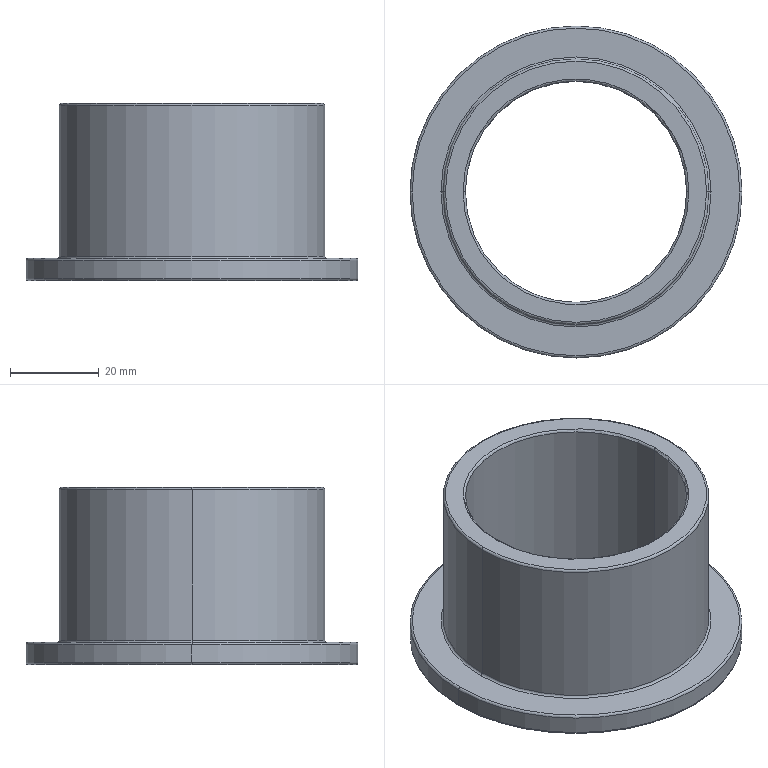Part | SolidWorks | features Fillet 3, Extrusion 1, ICE 1 | 1 solid | 21 faces | box 75 x 75 x 40 mm | volume 42442 mm3 | torus 12 | cylinder 6 | plane 3 | commonest cylinder face diameters 50 x2 60 x2 75 x2
STEP:
#1=CARTESIAN_POINT('',(37.,0.,0.));
#2=VERTEX_POINT('',#1);
#3=CARTESIAN_POINT('',(-37.,0.,0.));
#4=VERTEX_POINT('',#3);
#5=CARTESIAN_POINT('',(0.,0.,0.));
#6=DIRECTION('',(0.,0.,1.));
#7=DIRECTION('',(-1.,0.,0.));
#8=AXIS2_PLACEMENT_3D('',#5,#6,#7);
#9=CIRCLE('',#8,37.);
#10=EDGE_CURVE('',#2,#4,#9,.T.);
#11=ORIENTED_EDGE('',*,*,#10,.F.);
#12=CARTESIAN_POINT('',(37.5,0.,-0.5));
#13=VERTEX_POINT('',#12);
#14=CARTESIAN_POINT('',(37.,0.,-0.5));
#15=DIRECTION('',(0.,1.,0.));
#16=DIRECTION('',(-1.,0.,0.));
#17=AXIS2_PLACEMENT_3D('',#14,#15,#16);
#18=CIRCLE('',#17,0.5);
#19=EDGE_CURVE('',#2,#13,#18,.T.);
#20=ORIENTED_EDGE('',*,*,#19,.T.);
#21=CARTESIAN_POINT('',(-37.5,0.,-0.5));
#22=VERTEX_POINT('',#21);
#23=CARTESIAN_POINT('',(0.,0.,-0.5));
#24=DIRECTION('',(0.,0.,-1.));
#25=DIRECTION('',(-1.,0.,0.));
#26=AXIS2_PLACEMENT_3D('',#23,#24,#25);
#27=CIRCLE('',#26,37.5);
#28=EDGE_CURVE('',#22,#13,#27,.T.);
#29=ORIENTED_EDGE('',*,*,#28,.F.);
#30=CARTESIAN_POINT('',(-37.,0.,-0.5));
#31=DIRECTION('',(0.,-1.,0.));
#32=DIRECTION('',(0.,0.,-1.));
#33=AXIS2_PLACEMENT_3D('',#30,#31,#32);
#34=CIRCLE('',#33,0.5);
#35=EDGE_CURVE('',#4,#22,#34,.T.);
#36=ORIENTED_EDGE('',*,*,#35,.F.);
#37=EDGE_LOOP('',(#11,#20,#29,#36));
#38=FACE_OUTER_BOUND('',#37,.T.);
#39=CARTESIAN_POINT('',(0.,0.,-0.5));
#40=DIRECTION('',(0.,0.,-1.));
#41=DIRECTION('',(-1.,0.,0.));
#42=AXIS2_PLACEMENT_3D('',#39,#40,#41);
#43=TOROIDAL_SURFACE('',#42,37.,0.5);
#44=ADVANCED_FACE('',(#38),#43,.T.);
#45=CARTESIAN_POINT('',(37.5,0.,-4.5));
#46=VERTEX_POINT('',#45);
#47=CARTESIAN_POINT('',(-37.5,0.,-4.5));
#48=VERTEX_POINT('',#47);
#49=CARTESIAN_POINT('',(0.,0.,-4.5));
#50=DIRECTION('',(0.,0.,1.));
#51=DIRECTION('',(-1.,0.,0.));
#52=AXIS2_PLACEMENT_3D('',#49,#50,#51);
#53=CIRCLE('',#52,37.5);
#54=EDGE_CURVE('',#46,#48,#53,.T.);
#55=ORIENTED_EDGE('',*,*,#54,.F.);
#56=CARTESIAN_POINT('',(37.,0.,-5.));
#57=VERTEX_POINT('',#56);
#58=CARTESIAN_POINT('',(37.,0.,-4.5));
#59=DIRECTION('',(0.,1.,0.));
#60=DIRECTION('',(-1.,0.,0.));
#61=AXIS2_PLACEMENT_3D('',#58,#59,#60);
#62=CIRCLE('',#61,0.5);
#63=EDGE_CURVE('',#46,#57,#62,.T.);
#64=ORIENTED_EDGE('',*,*,#63,.T.);
#65=CARTESIAN_POINT('',(-37.,0.,-5.));
#66=VERTEX_POINT('',#65);
#67=CARTESIAN_POINT('',(0.,0.,-5.));
#68=DIRECTION('',(0.,0.,-1.));
#69=DIRECTION('',(-1.,0.,0.));
#70=AXIS2_PLACEMENT_3D('',#67,#68,#69);
#71=CIRCLE('',#70,37.);
#72=EDGE_CURVE('',#66,#57,#71,.T.);
#73=ORIENTED_EDGE('',*,*,#72,.F.);
#74=CARTESIAN_POINT('',(-37.,0.,-4.5));
#75=DIRECTION('',(0.,-1.,0.));
#76=DIRECTION('',(0.,0.,-1.));
#77=AXIS2_PLACEMENT_3D('',#74,#75,#76);
#78=CIRCLE('',#77,0.5);
#79=EDGE_CURVE('',#48,#66,#78,.T.);
#80=ORIENTED_EDGE('',*,*,#79,.F.);
#81=EDGE_LOOP('',(#55,#64,#73,#80));
#82=FACE_OUTER_BOUND('',#81,.T.);
#83=CARTESIAN_POINT('',(0.,0.,-4.5));
#84=DIRECTION('',(0.,0.,-1.));
#85=DIRECTION('',(-1.,0.,0.));
#86=AXIS2_PLACEMENT_3D('',#83,#84,#85);
#87=TOROIDAL_SURFACE('',#86,37.,0.5);
#88=ADVANCED_FACE('',(#82),#87,.T.);
#89=CARTESIAN_POINT('',(-30.,0.,34.5));
#90=VERTEX_POINT('',#89);
#91=CARTESIAN_POINT('',(30.,0.,34.5));
#92=VERTEX_POINT('',#91);
#93=CARTESIAN_POINT('',(0.,0.,34.5));
#94=DIRECTION('',(0.,0.,-1.));
#95=DIRECTION('',(1.,0.,0.));
#96=AXIS2_PLACEMENT_3D('',#93,#94,#95);
#97=CIRCLE('',#96,30.);
#98=EDGE_CURVE('',#90,#92,#97,.T.);
#99=ORIENTED_EDGE('',*,*,#98,.F.);
#100=CARTESIAN_POINT('',(-29.5,0.,35.));
#101=VERTEX_POINT('',#100);
#102=CARTESIAN_POINT('',(-29.5,0.,34.5));
#103=DIRECTION('',(0.,1.,0.));
#104=DIRECTION('',(-1.,0.,0.));
#105=AXIS2_PLACEMENT_3D('',#102,#103,#104);
#106=CIRCLE('',#105,0.5);
#107=EDGE_CURVE('',#90,#101,#106,.T.);
#108=ORIENTED_EDGE('',*,*,#107,.T.);
#109=CARTESIAN_POINT('',(29.5,0.,35.));
#110=VERTEX_POINT('',#109);
#111=CARTESIAN_POINT('',(0.,0.,35.));
#112=DIRECTION('',(0.,0.,1.));
#113=DIRECTION('',(1.,0.,0.));
#114=AXIS2_PLACEMENT_3D('',#111,#112,#113);
#115=CIRCLE('',#114,29.5);
#116=EDGE_CURVE('',#110,#101,#115,.T.);
#117=ORIENTED_EDGE('',*,*,#116,.F.);
#118=CARTESIAN_POINT('',(29.5,0.,34.5));
#119=DIRECTION('',(0.,-1.,0.));
#120=DIRECTION('',(0.,0.,-1.));
#121=AXIS2_PLACEMENT_3D('',#118,#119,#120);
#122=CIRCLE('',#121,0.5);
#123=EDGE_CURVE('',#92,#110,#122,.T.);
#124=ORIENTED_EDGE('',*,*,#123,.F.);
#125=EDGE_LOOP('',(#99,#108,#117,#124));
#126=FACE_OUTER_BOUND('',#125,.T.);
#127=CARTESIAN_POINT('',(0.,0.,34.5));
#128=DIRECTION('',(0.,0.,1.));
#129=DIRECTION('',(1.,0.,0.));
#130=AXIS2_PLACEMENT_3D('',#127,#128,#129);
#131=TOROIDAL_SURFACE('',#130,29.5,0.5);
#132=ADVANCED_FACE('',(#126),#131,.T.);
#133=CARTESIAN_POINT('',(-25.5,0.,35.));
#134=VERTEX_POINT('',#133);
#135=CARTESIAN_POINT('',(25.5,0.,35.));
#136=VERTEX_POINT('',#135);
#137=CARTESIAN_POINT('',(0.,0.,35.));
#138=DIRECTION('',(0.,0.,-1.));
#139=DIRECTION('',(1.,0.,0.));
#140=AXIS2_PLACEMENT_3D('',#137,#138,#139);
#141=CIRCLE('',#140,25.5);
#142=EDGE_CURVE('',#134,#136,#141,.T.);
#143=ORIENTED_EDGE('',*,*,#142,.F.);
#144=CARTESIAN_POINT('',(-25.,0.,34.5));
#145=VERTEX_POINT('',#144);
#146=CARTESIAN_POINT('',(-25.5,0.,34.5));
#147=DIRECTION('',(0.,1.,0.));
#148=DIRECTION('',(-1.,0.,0.));
#149=AXIS2_PLACEMENT_3D('',#146,#147,#148);
#150=CIRCLE('',#149,0.5);
#151=EDGE_CURVE('',#134,#145,#150,.T.);
#152=ORIENTED_EDGE('',*,*,#151,.T.);
#153=CARTESIAN_POINT('',(25.,0.,34.5));
#154=VERTEX_POINT('',#153);
#155=CARTESIAN_POINT('',(0.,0.,34.5));
#156=DIRECTION('',(0.,0.,1.));
#157=DIRECTION('',(1.,0.,0.));
#158=AXIS2_PLACEMENT_3D('',#155,#156,#157);
#159=CIRCLE('',#158,25.);
#160=EDGE_CURVE('',#154,#145,#159,.T.);
#161=ORIENTED_EDGE('',*,*,#160,.F.);
#162=CARTESIAN_POINT('',(25.5,0.,34.5));
#163=DIRECTION('',(0.,-1.,0.));
#164=DIRECTION('',(0.,0.,-1.));
#165=AXIS2_PLACEMENT_3D('',#162,#163,#164);
#166=CIRCLE('',#165,0.5);
#167=EDGE_CURVE('',#136,#154,#166,.T.);
#168=ORIENTED_EDGE('',*,*,#167,.F.);
#169=EDGE_LOOP('',(#143,#152,#161,#168));
#170=FACE_OUTER_BOUND('',#169,.T.);
#171=CARTESIAN_POINT('',(0.,0.,34.5));
#172=DIRECTION('',(0.,0.,1.));
#173=DIRECTION('',(1.,0.,0.));
#174=AXIS2_PLACEMENT_3D('',#171,#172,#173);
#175=TOROIDAL_SURFACE('',#174,25.5,0.5);
#176=ADVANCED_FACE('',(#170),#175,.T.);
#177=CARTESIAN_POINT('',(26.,0.,-5.));
#178=VERTEX_POINT('',#177);
#179=CARTESIAN_POINT('',(-26.,0.,-5.));
#180=VERTEX_POINT('',#179);
#181=CARTESIAN_POINT('',(0.,0.,-5.));
#182=DIRECTION('',(0.,0.,1.));
#183=DIRECTION('',(-1.,0.,0.));
#184=AXIS2_PLACEMENT_3D('',#181,#182,#183);
#185=CIRCLE('',#184,26.);
#186=EDGE_CURVE('',#178,#180,#185,.T.);
#187=ORIENTED_EDGE('',*,*,#186,.F.);
#188=CARTESIAN_POINT('',(25.,0.,-4.));
#189=VERTEX_POINT('',#188);
#190=CARTESIAN_POINT('',(26.,0.,-4.));
#191=DIRECTION('',(0.,1.,0.));
#192=DIRECTION('',(-1.,0.,0.));
#193=AXIS2_PLACEMENT_3D('',#190,#191,#192);
#194=CIRCLE('',#193,1.);
#195=EDGE_CURVE('',#178,#189,#194,.T.);
#196=ORIENTED_EDGE('',*,*,#195,.T.);
#197=CARTESIAN_POINT('',(-25.,0.,-4.));
#198=VERTEX_POINT('',#197);
#199=CARTESIAN_POINT('',(0.,0.,-4.));
#200=DIRECTION('',(0.,0.,-1.));
#201=DIRECTION('',(-1.,0.,0.));
#202=AXIS2_PLACEMENT_3D('',#199,#200,#201);
#203=CIRCLE('',#202,25.);
#204=EDGE_CURVE('',#198,#189,#203,.T.);
#205=ORIENTED_EDGE('',*,*,#204,.F.);
#206=CARTESIAN_POINT('',(-26.,0.,-4.));
#207=DIRECTION('',(0.,-1.,0.));
#208=DIRECTION('',(0.,0.,-1.));
#209=AXIS2_PLACEMENT_3D('',#206,#207,#208);
#210=CIRCLE('',#209,1.);
#211=EDGE_CURVE('',#180,#198,#210,.T.);
#212=ORIENTED_EDGE('',*,*,#211,.F.);
#213=EDGE_LOOP('',(#187,#196,#205,#212));
#214=FACE_OUTER_BOUND('',#213,.T.);
#215=CARTESIAN_POINT('',(0.,0.,-4.));
#216=DIRECTION('',(0.,0.,-1.));
#217=DIRECTION('',(-1.,0.,0.));
#218=AXIS2_PLACEMENT_3D('',#215,#216,#217);
#219=TOROIDAL_SURFACE('',#218,26.,1.);
#220=ADVANCED_FACE('',(#214),#219,.T.);
#221=CARTESIAN_POINT('',(30.5,0.,0.));
#222=VERTEX_POINT('',#221);
#223=CARTESIAN_POINT('',(-30.5,0.,0.));
#224=VERTEX_POINT('',#223);
#225=CARTESIAN_POINT('',(0.,0.,0.));
#226=DIRECTION('',(0.,0.,-1.));
#227=DIRECTION('',(-1.,0.,0.));
#228=AXIS2_PLACEMENT_3D('',#225,#226,#227);
#229=CIRCLE('',#228,30.5);
#230=EDGE_CURVE('',#222,#224,#229,.T.);
#231=ORIENTED_EDGE('',*,*,#230,.F.);
#232=CARTESIAN_POINT('',(30.,0.,0.5));
#233=VERTEX_POINT('',#232);
#234=CARTESIAN_POINT('',(30.5,0.,0.5));
#235=DIRECTION('',(0.,1.,0.));
#236=DIRECTION('',(-1.,0.,0.));
#237=AXIS2_PLACEMENT_3D('',#234,#235,#236);
#238=CIRCLE('',#237,0.5);
#239=EDGE_CURVE('',#222,#233,#238,.T.);
#240=ORIENTED_EDGE('',*,*,#239,.T.);
#241=CARTESIAN_POINT('',(-30.,0.,0.5));
#242=VERTEX_POINT('',#241);
#243=CARTESIAN_POINT('',(0.,0.,0.5));
#244=DIRECTION('',(0.,0.,1.));
#245=DIRECTION('',(-1.,0.,0.));
#246=AXIS2_PLACEMENT_3D('',#243,#244,#245);
#247=CIRCLE('',#246,30.);
#248=EDGE_CURVE('',#242,#233,#247,.T.);
#249=ORIENTED_EDGE('',*,*,#248,.F.);
#250=CARTESIAN_POINT('',(-30.5,0.,0.5));
#251=DIRECTION('',(0.,-1.,0.));
#252=DIRECTION('',(0.,0.,-1.));
#253=AXIS2_PLACEMENT_3D('',#250,#251,#252);
#254=CIRCLE('',#253,0.5);
#255=EDGE_CURVE('',#224,#242,#254,.T.);
#256=ORIENTED_EDGE('',*,*,#255,.F.);
#257=EDGE_LOOP('',(#231,#240,#249,#256));
#258=FACE_OUTER_BOUND('',#257,.T.);
#259=CARTESIAN_POINT('',(0.,0.,0.5));
#260=DIRECTION('',(0.,0.,-1.));
#261=DIRECTION('',(-1.,0.,0.));
#262=AXIS2_PLACEMENT_3D('',#259,#260,#261);
#263=TOROIDAL_SURFACE('',#262,30.5,0.5);
#264=ADVANCED_FACE('',(#258),#263,.F.);
#265=ORIENTED_EDGE('',*,*,#54,.T.);
#266=CARTESIAN_POINT('',(-37.5,0.,-5.));
#267=DIRECTION('',(0.,0.,1.));
#268=VECTOR('',#267,1000.);
#269=LINE('',#266,#268);
#270=EDGE_CURVE('',#48,#22,#269,.T.);
#271=ORIENTED_EDGE('',*,*,#270,.T.);
#272=ORIENTED_EDGE('',*,*,#28,.T.);
#273=CARTESIAN_POINT('',(37.5,0.,-5.));
#274=DIRECTION('',(0.,0.,1.));
#275=VECTOR('',#274,1000.);
#276=LINE('',#273,#275);
#277=EDGE_CURVE('',#46,#13,#276,.T.);
#278=ORIENTED_EDGE('',*,*,#277,.F.);
#279=EDGE_LOOP('',(#265,#271,#272,#278));
#280=FACE_OUTER_BOUND('',#279,.T.);
#281=CARTESIAN_POINT('',(0.,0.,-5.));
#282=DIRECTION('',(0.,0.,1.));
#283=DIRECTION('',(1.,0.,0.));
#284=AXIS2_PLACEMENT_3D('',#281,#282,#283);
#285=CYLINDRICAL_SURFACE('',#284,37.5);
#286=ADVANCED_FACE('',(#280),#285,.T.);
#287=CARTESIAN_POINT('',(0.,0.,34.5));
#288=DIRECTION('',(0.,0.,1.));
#289=DIRECTION('',(1.,0.,0.));
#290=AXIS2_PLACEMENT_3D('',#287,#288,#289);
#291=CIRCLE('',#290,25.);
#292=EDGE_CURVE('',#145,#154,#291,.T.);
#293=ORIENTED_EDGE('',*,*,#292,.T.);
#294=CARTESIAN_POINT('',(25.,0.,35.));
#295=DIRECTION('',(0.,0.,-1.));
#296=VECTOR('',#295,1000.);
#297=LINE('',#294,#296);
#298=EDGE_CURVE('',#154,#189,#297,.T.);
#299=ORIENTED_EDGE('',*,*,#298,.T.);
#300=CARTESIAN_POINT('',(0.,0.,-4.));
#301=DIRECTION('',(0.,0.,-1.));
#302=DIRECTION('',(-1.,0.,0.));
#303=AXIS2_PLACEMENT_3D('',#300,#301,#302);
#304=CIRCLE('',#303,25.);
#305=EDGE_CURVE('',#189,#198,#304,.T.);
#306=ORIENTED_EDGE('',*,*,#305,.T.);
#307=CARTESIAN_POINT('',(-25.,0.,35.));
#308=DIRECTION('',(0.,0.,-1.));
#309=VECTOR('',#308,1000.);
#310=LINE('',#307,#309);
#311=EDGE_CURVE('',#145,#198,#310,.T.);
#312=ORIENTED_EDGE('',*,*,#311,.F.);
#313=EDGE_LOOP('',(#293,#299,#306,#312));
#314=FACE_OUTER_BOUND('',#313,.T.);
#315=CARTESIAN_POINT('',(0.,0.,35.));
#316=DIRECTION('',(0.,0.,-1.));
#317=DIRECTION('',(-1.,0.,0.));
#318=AXIS2_PLACEMENT_3D('',#315,#316,#317);
#319=CYLINDRICAL_SURFACE('',#318,25.);
#320=ADVANCED_FACE('',(#314),#319,.F.);
#321=ORIENTED_EDGE('',*,*,#98,.T.);
#322=CARTESIAN_POINT('',(30.,0.,35.));
#323=DIRECTION('',(0.,0.,-1.));
#324=VECTOR('',#323,1000.);
#325=LINE('',#322,#324);
#326=EDGE_CURVE('',#92,#233,#325,.T.);
#327=ORIENTED_EDGE('',*,*,#326,.T.);
#328=CARTESIAN_POINT('',(0.,0.,0.5));
#329=DIRECTION('',(0.,0.,1.));
#330=DIRECTION('',(-1.,0.,0.));
#331=AXIS2_PLACEMENT_3D('',#328,#329,#330);
#332=CIRCLE('',#331,30.);
#333=EDGE_CURVE('',#233,#242,#332,.T.);
#334=ORIENTED_EDGE('',*,*,#333,.T.);
#335=CARTESIAN_POINT('',(-30.,0.,35.));
#336=DIRECTION('',(0.,0.,-1.));
#337=VECTOR('',#336,1000.);
#338=LINE('',#335,#337);
#339=EDGE_CURVE('',#90,#242,#338,.T.);
#340=ORIENTED_EDGE('',*,*,#339,.F.);
#341=EDGE_LOOP('',(#321,#327,#334,#340));
#342=FACE_OUTER_BOUND('',#341,.T.);
#343=CARTESIAN_POINT('',(0.,0.,35.));
#344=DIRECTION('',(0.,0.,-1.));
#345=DIRECTION('',(-1.,0.,0.));
#346=AXIS2_PLACEMENT_3D('',#343,#344,#345);
#347=CYLINDRICAL_SURFACE('',#346,30.);
#348=ADVANCED_FACE('',(#342),#347,.T.);
#349=CARTESIAN_POINT('',(0.,0.,35.));
#350=DIRECTION('',(0.,0.,-1.));
#351=DIRECTION('',(1.,0.,0.));
#352=AXIS2_PLACEMENT_3D('',#349,#350,#351);
#353=CIRCLE('',#352,25.5);
#354=EDGE_CURVE('',#136,#134,#353,.T.);
#355=ORIENTED_EDGE('',*,*,#354,.T.);
#356=ORIENTED_EDGE('',*,*,#142,.T.);
#357=EDGE_LOOP('',(#355,#356));
#358=FACE_BOUND('',#357,.T.);
#359=ORIENTED_EDGE('',*,*,#116,.T.);
#360=CARTESIAN_POINT('',(0.,0.,35.));
#361=DIRECTION('',(0.,0.,1.));
#362=DIRECTION('',(1.,0.,0.));
#363=AXIS2_PLACEMENT_3D('',#360,#361,#362);
#364=CIRCLE('',#363,29.5);
#365=EDGE_CURVE('',#101,#110,#364,.T.);
#366=ORIENTED_EDGE('',*,*,#365,.T.);
#367=EDGE_LOOP('',(#359,#366));
#368=FACE_OUTER_BOUND('',#367,.T.);
#369=CARTESIAN_POINT('',(0.,0.,35.));
#370=DIRECTION('',(0.,0.,1.));
#371=DIRECTION('',(1.,0.,0.));
#372=AXIS2_PLACEMENT_3D('',#369,#370,#371);
#373=PLANE('',#372);
#374=ADVANCED_FACE('',(#358,#368),#373,.T.);
#375=ORIENTED_EDGE('',*,*,#326,.F.);
#376=CARTESIAN_POINT('',(0.,0.,34.5));
#377=DIRECTION('',(0.,0.,-1.));
#378=DIRECTION('',(1.,0.,0.));
#379=AXIS2_PLACEMENT_3D('',#376,#377,#378);
#380=CIRCLE('',#379,30.);
#381=EDGE_CURVE('',#92,#90,#380,.T.);
#382=ORIENTED_EDGE('',*,*,#381,.T.);
#383=ORIENTED_EDGE('',*,*,#339,.T.);
#384=ORIENTED_EDGE('',*,*,#248,.T.);
#385=EDGE_LOOP('',(#375,#382,#383,#384));
#386=FACE_OUTER_BOUND('',#385,.T.);
#387=CARTESIAN_POINT('',(0.,0.,35.));
#388=DIRECTION('',(0.,0.,-1.));
#389=DIRECTION('',(-1.,0.,0.));
#390=AXIS2_PLACEMENT_3D('',#387,#388,#389);
#391=CYLINDRICAL_SURFACE('',#390,30.);
#392=ADVANCED_FACE('',(#386),#391,.T.);
#393=ORIENTED_EDGE('',*,*,#298,.F.);
#394=ORIENTED_EDGE('',*,*,#160,.T.);
#395=ORIENTED_EDGE('',*,*,#311,.T.);
#396=ORIENTED_EDGE('',*,*,#204,.T.);
#397=EDGE_LOOP('',(#393,#394,#395,#396));
#398=FACE_OUTER_BOUND('',#397,.T.);
#399=CARTESIAN_POINT('',(0.,0.,35.));
#400=DIRECTION('',(0.,0.,-1.));
#401=DIRECTION('',(-1.,0.,0.));
#402=AXIS2_PLACEMENT_3D('',#399,#400,#401);
#403=CYLINDRICAL_SURFACE('',#402,25.);
#404=ADVANCED_FACE('',(#398),#403,.F.);
#405=ORIENTED_EDGE('',*,*,#72,.T.);
#406=CARTESIAN_POINT('',(0.,0.,-5.));
#407=DIRECTION('',(0.,0.,-1.));
#408=DIRECTION('',(-1.,0.,0.));
#409=AXIS2_PLACEMENT_3D('',#406,#407,#408);
#410=CIRCLE('',#409,37.);
#411=EDGE_CURVE('',#57,#66,#410,.T.);
#412=ORIENTED_EDGE('',*,*,#411,.T.);
#413=EDGE_LOOP('',(#405,#412));
#414=FACE_OUTER_BOUND('',#413,.T.);
#415=CARTESIAN_POINT('',(0.,0.,-5.));
#416=DIRECTION('',(0.,0.,1.));
#417=DIRECTION('',(-1.,0.,0.));
#418=AXIS2_PLACEMENT_3D('',#415,#416,#417);
#419=CIRCLE('',#418,26.);
#420=EDGE_CURVE('',#180,#178,#419,.T.);
#421=ORIENTED_EDGE('',*,*,#420,.T.);
#422=ORIENTED_EDGE('',*,*,#186,.T.);
#423=EDGE_LOOP('',(#421,#422));
#424=FACE_BOUND('',#423,.T.);
#425=CARTESIAN_POINT('',(0.,0.,-5.));
#426=DIRECTION('',(0.,0.,-1.));
#427=DIRECTION('',(-1.,0.,0.));
#428=AXIS2_PLACEMENT_3D('',#425,#426,#427);
#429=PLANE('',#428);
#430=ADVANCED_FACE('',(#414,#424),#429,.T.);
#431=CARTESIAN_POINT('',(0.,0.,0.));
#432=DIRECTION('',(0.,0.,1.));
#433=DIRECTION('',(-1.,0.,0.));
#434=AXIS2_PLACEMENT_3D('',#431,#432,#433);
#435=CIRCLE('',#434,37.);
#436=EDGE_CURVE('',#4,#2,#435,.T.);
#437=ORIENTED_EDGE('',*,*,#436,.T.);
#438=ORIENTED_EDGE('',*,*,#10,.T.);
#439=EDGE_LOOP('',(#437,#438));
#440=FACE_OUTER_BOUND('',#439,.T.);
#441=CARTESIAN_POINT('',(0.,0.,0.));
#442=DIRECTION('',(0.,0.,-1.));
#443=DIRECTION('',(-1.,0.,0.));
#444=AXIS2_PLACEMENT_3D('',#441,#442,#443);
#445=CIRCLE('',#444,30.5);
#446=EDGE_CURVE('',#224,#222,#445,.T.);
#447=ORIENTED_EDGE('',*,*,#446,.T.);
#448=ORIENTED_EDGE('',*,*,#230,.T.);
#449=EDGE_LOOP('',(#447,#448));
#450=FACE_BOUND('',#449,.T.);
#451=CARTESIAN_POINT('',(0.,0.,0.));
#452=DIRECTION('',(0.,0.,-1.));
#453=DIRECTION('',(-1.,0.,0.));
#454=AXIS2_PLACEMENT_3D('',#451,#452,#453);
#455=PLANE('',#454);
#456=ADVANCED_FACE('',(#440,#450),#455,.F.);
#457=ORIENTED_EDGE('',*,*,#270,.F.);
#458=CARTESIAN_POINT('',(0.,0.,-4.5));
#459=DIRECTION('',(0.,0.,1.));
#460=DIRECTION('',(-1.,0.,0.));
#461=AXIS2_PLACEMENT_3D('',#458,#459,#460);
#462=CIRCLE('',#461,37.5);
#463=EDGE_CURVE('',#48,#46,#462,.T.);
#464=ORIENTED_EDGE('',*,*,#463,.T.);
#465=ORIENTED_EDGE('',*,*,#277,.T.);
#466=CARTESIAN_POINT('',(0.,0.,-0.5));
#467=DIRECTION('',(0.,0.,-1.));
#468=DIRECTION('',(-1.,0.,0.));
#469=AXIS2_PLACEMENT_3D('',#466,#467,#468);
#470=CIRCLE('',#469,37.5);
#471=EDGE_CURVE('',#13,#22,#470,.T.);
#472=ORIENTED_EDGE('',*,*,#471,.T.);
#473=EDGE_LOOP('',(#457,#464,#465,#472));
#474=FACE_OUTER_BOUND('',#473,.T.);
#475=CARTESIAN_POINT('',(0.,0.,-5.));
#476=DIRECTION('',(0.,0.,1.));
#477=DIRECTION('',(1.,0.,0.));
#478=AXIS2_PLACEMENT_3D('',#475,#476,#477);
#479=CYLINDRICAL_SURFACE('',#478,37.5);
#480=ADVANCED_FACE('',(#474),#479,.T.);
#481=ORIENTED_EDGE('',*,*,#239,.F.);
#482=ORIENTED_EDGE('',*,*,#446,.F.);
#483=ORIENTED_EDGE('',*,*,#255,.T.);
#484=ORIENTED_EDGE('',*,*,#333,.F.);
#485=EDGE_LOOP('',(#481,#482,#483,#484));
#486=FACE_OUTER_BOUND('',#485,.T.);
#487=CARTESIAN_POINT('',(0.,0.,0.5));
#488=DIRECTION('',(0.,0.,-1.));
#489=DIRECTION('',(-1.,0.,0.));
#490=AXIS2_PLACEMENT_3D('',#487,#488,#489);
#491=TOROIDAL_SURFACE('',#490,30.5,0.5);
#492=ADVANCED_FACE('',(#486),#491,.F.);
#493=ORIENTED_EDGE('',*,*,#195,.F.);
#494=ORIENTED_EDGE('',*,*,#420,.F.);
#495=ORIENTED_EDGE('',*,*,#211,.T.);
#496=ORIENTED_EDGE('',*,*,#305,.F.);
#497=EDGE_LOOP('',(#493,#494,#495,#496));
#498=FACE_OUTER_BOUND('',#497,.T.);
#499=CARTESIAN_POINT('',(0.,0.,-4.));
#500=DIRECTION('',(0.,0.,-1.));
#501=DIRECTION('',(-1.,0.,0.));
#502=AXIS2_PLACEMENT_3D('',#499,#500,#501);
#503=TOROIDAL_SURFACE('',#502,26.,1.);
#504=ADVANCED_FACE('',(#498),#503,.T.);
#505=ORIENTED_EDGE('',*,*,#151,.F.);
#506=ORIENTED_EDGE('',*,*,#354,.F.);
#507=ORIENTED_EDGE('',*,*,#167,.T.);
#508=ORIENTED_EDGE('',*,*,#292,.F.);
#509=EDGE_LOOP('',(#505,#506,#507,#508));
#510=FACE_OUTER_BOUND('',#509,.T.);
#511=CARTESIAN_POINT('',(0.,0.,34.5));
#512=DIRECTION('',(0.,0.,1.));
#513=DIRECTION('',(1.,0.,0.));
#514=AXIS2_PLACEMENT_3D('',#511,#512,#513);
#515=TOROIDAL_SURFACE('',#514,25.5,0.5);
#516=ADVANCED_FACE('',(#510),#515,.T.);
#517=ORIENTED_EDGE('',*,*,#107,.F.);
#518=ORIENTED_EDGE('',*,*,#381,.F.);
#519=ORIENTED_EDGE('',*,*,#123,.T.);
#520=ORIENTED_EDGE('',*,*,#365,.F.);
#521=EDGE_LOOP('',(#517,#518,#519,#520));
#522=FACE_OUTER_BOUND('',#521,.T.);
#523=CARTESIAN_POINT('',(0.,0.,34.5));
#524=DIRECTION('',(0.,0.,1.));
#525=DIRECTION('',(1.,0.,0.));
#526=AXIS2_PLACEMENT_3D('',#523,#524,#525);
#527=TOROIDAL_SURFACE('',#526,29.5,0.5);
#528=ADVANCED_FACE('',(#522),#527,.T.);
#529=ORIENTED_EDGE('',*,*,#63,.F.);
#530=ORIENTED_EDGE('',*,*,#463,.F.);
#531=ORIENTED_EDGE('',*,*,#79,.T.);
#532=ORIENTED_EDGE('',*,*,#411,.F.);
#533=EDGE_LOOP('',(#529,#530,#531,#532));
#534=FACE_OUTER_BOUND('',#533,.T.);
#535=CARTESIAN_POINT('',(0.,0.,-4.5));
#536=DIRECTION('',(0.,0.,-1.));
#537=DIRECTION('',(-1.,0.,0.));
#538=AXIS2_PLACEMENT_3D('',#535,#536,#537);
#539=TOROIDAL_SURFACE('',#538,37.,0.5);
#540=ADVANCED_FACE('',(#534),#539,.T.);
#541=ORIENTED_EDGE('',*,*,#19,.F.);
#542=ORIENTED_EDGE('',*,*,#436,.F.);
#543=ORIENTED_EDGE('',*,*,#35,.T.);
#544=ORIENTED_EDGE('',*,*,#471,.F.);
#545=EDGE_LOOP('',(#541,#542,#543,#544));
#546=FACE_OUTER_BOUND('',#545,.T.);
#547=CARTESIAN_POINT('',(0.,0.,-0.5));
#548=DIRECTION('',(0.,0.,-1.));
#549=DIRECTION('',(-1.,0.,0.));
#550=AXIS2_PLACEMENT_3D('',#547,#548,#549);
#551=TOROIDAL_SURFACE('',#550,37.,0.5);
#552=ADVANCED_FACE('',(#546),#551,.T.);
#553=CLOSED_SHELL('',(#44,#88,#132,#176,#220,#264,#286,#320,#348,#374,#392,#404,#430,#456,#480,#492,#504,#516,#528,#540,#552));
#554=MANIFOLD_SOLID_BREP('',#553);
#555=CARTESIAN_POINT('',(0.,0.,0.));
#556=DIRECTION('',(0.,0.,1.));
#557=DIRECTION('',(1.,0.,0.));
#558=AXIS2_PLACEMENT_3D('',#555,#556,#557);
#559=(LENGTH_UNIT()NAMED_UNIT(*)SI_UNIT(.MILLI.,.METRE.));
#560=UNCERTAINTY_MEASURE_WITH_UNIT(LENGTH_MEASURE(0.00001),#559,'','');
#561=(NAMED_UNIT(*)PLANE_ANGLE_UNIT()SI_UNIT($,.RADIAN.));
#562=(NAMED_UNIT(*)SI_UNIT($,.STERADIAN.)SOLID_ANGLE_UNIT());
#563=(GEOMETRIC_REPRESENTATION_CONTEXT(3)GLOBAL_UNCERTAINTY_ASSIGNED_CONTEXT((#560))GLOBAL_UNIT_ASSIGNED_CONTEXT((#559,#561,#562))REPRESENTATION_CONTEXT('',''));
#564=ADVANCED_BREP_SHAPE_REPRESENTATION('',(#554,#558),#563);